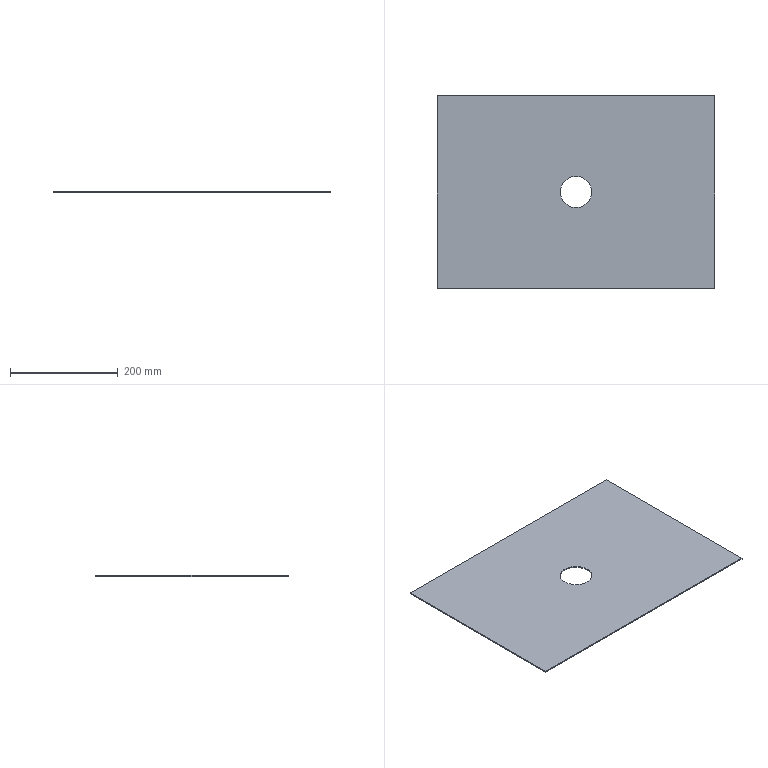Part | SolidWorks | features BaseBody 1 | 1 solid | 8 faces | box 514.4 x 356.4 x 2 mm | volume 361307 mm3 | plane 6 | cylinder 2 | commonest cylinder face diameters 58.4 x2
STEP:
#1=CARTESIAN_POINT('',(29.2,0.,10.5));
#2=VERTEX_POINT('',#1);
#3=CARTESIAN_POINT('',(-29.2,0.,10.5));
#4=VERTEX_POINT('',#3);
#5=CARTESIAN_POINT('',(0.,0.,10.5));
#6=DIRECTION('',(0.,0.,-1.));
#7=DIRECTION('',(-1.,0.,0.));
#8=AXIS2_PLACEMENT_3D('',#5,#6,#7);
#9=CIRCLE('',#8,29.2);
#10=EDGE_CURVE('',#2,#4,#9,.T.);
#11=ORIENTED_EDGE('',*,*,#10,.F.);
#12=CARTESIAN_POINT('',(29.2,0.,8.5));
#13=VERTEX_POINT('',#12);
#14=CARTESIAN_POINT('',(29.2,0.,10.5));
#15=DIRECTION('',(0.,0.,-1.));
#16=VECTOR('',#15,1000.);
#17=LINE('',#14,#16);
#18=EDGE_CURVE('',#2,#13,#17,.T.);
#19=ORIENTED_EDGE('',*,*,#18,.T.);
#20=CARTESIAN_POINT('',(-29.2,0.,8.5));
#21=VERTEX_POINT('',#20);
#22=CARTESIAN_POINT('',(0.,0.,8.5));
#23=DIRECTION('',(0.,0.,1.));
#24=DIRECTION('',(-1.,0.,0.));
#25=AXIS2_PLACEMENT_3D('',#22,#23,#24);
#26=CIRCLE('',#25,29.2);
#27=EDGE_CURVE('',#21,#13,#26,.T.);
#28=ORIENTED_EDGE('',*,*,#27,.F.);
#29=CARTESIAN_POINT('',(-29.2,0.,10.5));
#30=DIRECTION('',(0.,0.,-1.));
#31=VECTOR('',#30,1000.);
#32=LINE('',#29,#31);
#33=EDGE_CURVE('',#4,#21,#32,.T.);
#34=ORIENTED_EDGE('',*,*,#33,.F.);
#35=EDGE_LOOP('',(#11,#19,#28,#34));
#36=FACE_OUTER_BOUND('',#35,.T.);
#37=CARTESIAN_POINT('',(0.,0.,10.5));
#38=DIRECTION('',(0.,0.,-1.));
#39=DIRECTION('',(-1.,0.,0.));
#40=AXIS2_PLACEMENT_3D('',#37,#38,#39);
#41=CYLINDRICAL_SURFACE('',#40,29.2);
#42=ADVANCED_FACE('',(#36),#41,.F.);
#43=ORIENTED_EDGE('',*,*,#27,.T.);
#44=CARTESIAN_POINT('',(0.,0.,8.5));
#45=DIRECTION('',(0.,0.,1.));
#46=DIRECTION('',(-1.,0.,0.));
#47=AXIS2_PLACEMENT_3D('',#44,#45,#46);
#48=CIRCLE('',#47,29.2);
#49=EDGE_CURVE('',#13,#21,#48,.T.);
#50=ORIENTED_EDGE('',*,*,#49,.T.);
#51=EDGE_LOOP('',(#43,#50));
#52=FACE_BOUND('',#51,.T.);
#53=CARTESIAN_POINT('',(257.2,-178.2,8.5));
#54=VERTEX_POINT('',#53);
#55=CARTESIAN_POINT('',(-257.2,-178.2,8.5));
#56=VERTEX_POINT('',#55);
#57=CARTESIAN_POINT('',(0.,-178.2,8.5));
#58=DIRECTION('',(-1.,0.,0.));
#59=VECTOR('',#58,1000.);
#60=LINE('',#57,#59);
#61=EDGE_CURVE('',#54,#56,#60,.T.);
#62=ORIENTED_EDGE('',*,*,#61,.T.);
#63=CARTESIAN_POINT('',(-257.2,178.2,8.5));
#64=VERTEX_POINT('',#63);
#65=CARTESIAN_POINT('',(-257.2,0.,8.5));
#66=DIRECTION('',(0.,1.,0.));
#67=VECTOR('',#66,1000.);
#68=LINE('',#65,#67);
#69=EDGE_CURVE('',#56,#64,#68,.T.);
#70=ORIENTED_EDGE('',*,*,#69,.T.);
#71=CARTESIAN_POINT('',(257.2,178.2,8.5));
#72=VERTEX_POINT('',#71);
#73=CARTESIAN_POINT('',(0.,178.2,8.5));
#74=DIRECTION('',(1.,0.,0.));
#75=VECTOR('',#74,1000.);
#76=LINE('',#73,#75);
#77=EDGE_CURVE('',#64,#72,#76,.T.);
#78=ORIENTED_EDGE('',*,*,#77,.T.);
#79=CARTESIAN_POINT('',(257.2,0.,8.5));
#80=DIRECTION('',(0.,-1.,0.));
#81=VECTOR('',#80,1000.);
#82=LINE('',#79,#81);
#83=EDGE_CURVE('',#72,#54,#82,.T.);
#84=ORIENTED_EDGE('',*,*,#83,.T.);
#85=EDGE_LOOP('',(#62,#70,#78,#84));
#86=FACE_OUTER_BOUND('',#85,.T.);
#87=CARTESIAN_POINT('',(0.,0.,8.5));
#88=DIRECTION('',(0.,0.,-1.));
#89=DIRECTION('',(-1.,0.,0.));
#90=AXIS2_PLACEMENT_3D('',#87,#88,#89);
#91=PLANE('',#90);
#92=ADVANCED_FACE('',(#52,#86),#91,.T.);
#93=ORIENTED_EDGE('',*,*,#18,.F.);
#94=CARTESIAN_POINT('',(0.,0.,10.5));
#95=DIRECTION('',(0.,0.,-1.));
#96=DIRECTION('',(-1.,0.,0.));
#97=AXIS2_PLACEMENT_3D('',#94,#95,#96);
#98=CIRCLE('',#97,29.2);
#99=EDGE_CURVE('',#4,#2,#98,.T.);
#100=ORIENTED_EDGE('',*,*,#99,.F.);
#101=ORIENTED_EDGE('',*,*,#33,.T.);
#102=ORIENTED_EDGE('',*,*,#49,.F.);
#103=EDGE_LOOP('',(#93,#100,#101,#102));
#104=FACE_OUTER_BOUND('',#103,.T.);
#105=CARTESIAN_POINT('',(0.,0.,10.5));
#106=DIRECTION('',(0.,0.,-1.));
#107=DIRECTION('',(-1.,0.,0.));
#108=AXIS2_PLACEMENT_3D('',#105,#106,#107);
#109=CYLINDRICAL_SURFACE('',#108,29.2);
#110=ADVANCED_FACE('',(#104),#109,.F.);
#111=ORIENTED_EDGE('',*,*,#69,.F.);
#112=CARTESIAN_POINT('',(-257.2,-178.2,10.5));
#113=VERTEX_POINT('',#112);
#114=CARTESIAN_POINT('',(-257.2,-178.2,10.5));
#115=DIRECTION('',(0.,0.,1.));
#116=VECTOR('',#115,1000.);
#117=LINE('',#114,#116);
#118=EDGE_CURVE('',#56,#113,#117,.T.);
#119=ORIENTED_EDGE('',*,*,#118,.T.);
#120=CARTESIAN_POINT('',(-257.2,178.2,10.5));
#121=VERTEX_POINT('',#120);
#122=CARTESIAN_POINT('',(-257.2,-178.2,10.5));
#123=DIRECTION('',(0.,1.,0.));
#124=VECTOR('',#123,1000.);
#125=LINE('',#122,#124);
#126=EDGE_CURVE('',#113,#121,#125,.T.);
#127=ORIENTED_EDGE('',*,*,#126,.T.);
#128=CARTESIAN_POINT('',(-257.2,178.2,10.5));
#129=DIRECTION('',(0.,0.,-1.));
#130=VECTOR('',#129,1000.);
#131=LINE('',#128,#130);
#132=EDGE_CURVE('',#121,#64,#131,.T.);
#133=ORIENTED_EDGE('',*,*,#132,.T.);
#134=EDGE_LOOP('',(#111,#119,#127,#133));
#135=FACE_OUTER_BOUND('',#134,.T.);
#136=CARTESIAN_POINT('',(-257.2,-178.2,10.5));
#137=DIRECTION('',(-1.,0.,0.));
#138=DIRECTION('',(0.,-1.,0.));
#139=AXIS2_PLACEMENT_3D('',#136,#137,#138);
#140=PLANE('',#139);
#141=ADVANCED_FACE('',(#135),#140,.T.);
#142=ORIENTED_EDGE('',*,*,#61,.F.);
#143=CARTESIAN_POINT('',(257.2,-178.2,10.5));
#144=VERTEX_POINT('',#143);
#145=CARTESIAN_POINT('',(257.2,-178.2,10.5));
#146=DIRECTION('',(0.,0.,1.));
#147=VECTOR('',#146,1000.);
#148=LINE('',#145,#147);
#149=EDGE_CURVE('',#54,#144,#148,.T.);
#150=ORIENTED_EDGE('',*,*,#149,.T.);
#151=CARTESIAN_POINT('',(257.2,-178.2,10.5));
#152=DIRECTION('',(-1.,0.,0.));
#153=VECTOR('',#152,1000.);
#154=LINE('',#151,#153);
#155=EDGE_CURVE('',#144,#113,#154,.T.);
#156=ORIENTED_EDGE('',*,*,#155,.T.);
#157=ORIENTED_EDGE('',*,*,#118,.F.);
#158=EDGE_LOOP('',(#142,#150,#156,#157));
#159=FACE_OUTER_BOUND('',#158,.T.);
#160=CARTESIAN_POINT('',(257.2,-178.2,10.5));
#161=DIRECTION('',(0.,-1.,0.));
#162=DIRECTION('',(0.,0.,-1.));
#163=AXIS2_PLACEMENT_3D('',#160,#161,#162);
#164=PLANE('',#163);
#165=ADVANCED_FACE('',(#159),#164,.T.);
#166=ORIENTED_EDGE('',*,*,#83,.F.);
#167=CARTESIAN_POINT('',(257.2,178.2,10.5));
#168=VERTEX_POINT('',#167);
#169=CARTESIAN_POINT('',(257.2,178.2,10.5));
#170=DIRECTION('',(0.,0.,1.));
#171=VECTOR('',#170,1000.);
#172=LINE('',#169,#171);
#173=EDGE_CURVE('',#72,#168,#172,.T.);
#174=ORIENTED_EDGE('',*,*,#173,.T.);
#175=CARTESIAN_POINT('',(257.2,178.2,10.5));
#176=DIRECTION('',(0.,-1.,0.));
#177=VECTOR('',#176,1000.);
#178=LINE('',#175,#177);
#179=EDGE_CURVE('',#168,#144,#178,.T.);
#180=ORIENTED_EDGE('',*,*,#179,.T.);
#181=ORIENTED_EDGE('',*,*,#149,.F.);
#182=EDGE_LOOP('',(#166,#174,#180,#181));
#183=FACE_OUTER_BOUND('',#182,.T.);
#184=CARTESIAN_POINT('',(257.2,178.2,10.5));
#185=DIRECTION('',(1.,0.,0.));
#186=DIRECTION('',(0.,0.,-1.));
#187=AXIS2_PLACEMENT_3D('',#184,#185,#186);
#188=PLANE('',#187);
#189=ADVANCED_FACE('',(#183),#188,.T.);
#190=ORIENTED_EDGE('',*,*,#77,.F.);
#191=ORIENTED_EDGE('',*,*,#132,.F.);
#192=CARTESIAN_POINT('',(-257.2,178.2,10.5));
#193=DIRECTION('',(1.,0.,0.));
#194=VECTOR('',#193,1000.);
#195=LINE('',#192,#194);
#196=EDGE_CURVE('',#121,#168,#195,.T.);
#197=ORIENTED_EDGE('',*,*,#196,.T.);
#198=ORIENTED_EDGE('',*,*,#173,.F.);
#199=EDGE_LOOP('',(#190,#191,#197,#198));
#200=FACE_OUTER_BOUND('',#199,.T.);
#201=CARTESIAN_POINT('',(-257.2,178.2,10.5));
#202=DIRECTION('',(0.,1.,0.));
#203=DIRECTION('',(-1.,0.,0.));
#204=AXIS2_PLACEMENT_3D('',#201,#202,#203);
#205=PLANE('',#204);
#206=ADVANCED_FACE('',(#200),#205,.T.);
#207=ORIENTED_EDGE('',*,*,#99,.T.);
#208=ORIENTED_EDGE('',*,*,#10,.T.);
#209=EDGE_LOOP('',(#207,#208));
#210=FACE_BOUND('',#209,.T.);
#211=ORIENTED_EDGE('',*,*,#126,.F.);
#212=ORIENTED_EDGE('',*,*,#155,.F.);
#213=ORIENTED_EDGE('',*,*,#179,.F.);
#214=ORIENTED_EDGE('',*,*,#196,.F.);
#215=EDGE_LOOP('',(#211,#212,#213,#214));
#216=FACE_OUTER_BOUND('',#215,.T.);
#217=CARTESIAN_POINT('',(0.,0.,10.5));
#218=DIRECTION('',(0.,0.,-1.));
#219=DIRECTION('',(-1.,0.,0.));
#220=AXIS2_PLACEMENT_3D('',#217,#218,#219);
#221=PLANE('',#220);
#222=ADVANCED_FACE('',(#210,#216),#221,.F.);
#223=CLOSED_SHELL('',(#42,#92,#110,#141,#165,#189,#206,#222));
#224=MANIFOLD_SOLID_BREP('',#223);
#225=CARTESIAN_POINT('',(0.,0.,0.));
#226=DIRECTION('',(0.,0.,1.));
#227=DIRECTION('',(1.,0.,0.));
#228=AXIS2_PLACEMENT_3D('',#225,#226,#227);
#229=(LENGTH_UNIT()NAMED_UNIT(*)SI_UNIT(.MILLI.,.METRE.));
#230=UNCERTAINTY_MEASURE_WITH_UNIT(LENGTH_MEASURE(0.00001),#229,'','');
#231=(NAMED_UNIT(*)PLANE_ANGLE_UNIT()SI_UNIT($,.RADIAN.));
#232=(NAMED_UNIT(*)SI_UNIT($,.STERADIAN.)SOLID_ANGLE_UNIT());
#233=(GEOMETRIC_REPRESENTATION_CONTEXT(3)GLOBAL_UNCERTAINTY_ASSIGNED_CONTEXT((#230))GLOBAL_UNIT_ASSIGNED_CONTEXT((#229,#231,#232))REPRESENTATION_CONTEXT('',''));
#234=ADVANCED_BREP_SHAPE_REPRESENTATION('',(#224,#228),#233);